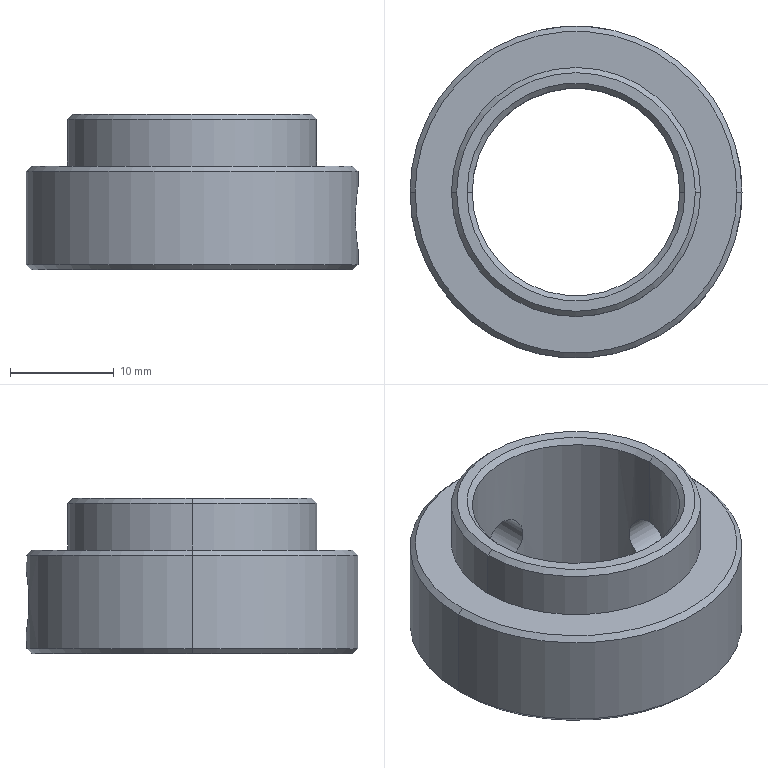Part | STEP file | 0229_Z_SCSBS20-24_1 | 1 solid | 27 faces | box 32 x 32 x 15 mm | volume 5310 mm3 | cone 14 | cylinder 10 | plane 3 | commonest cylinder face diameters 4.917 x4 20 x2 24 x2 32 x2